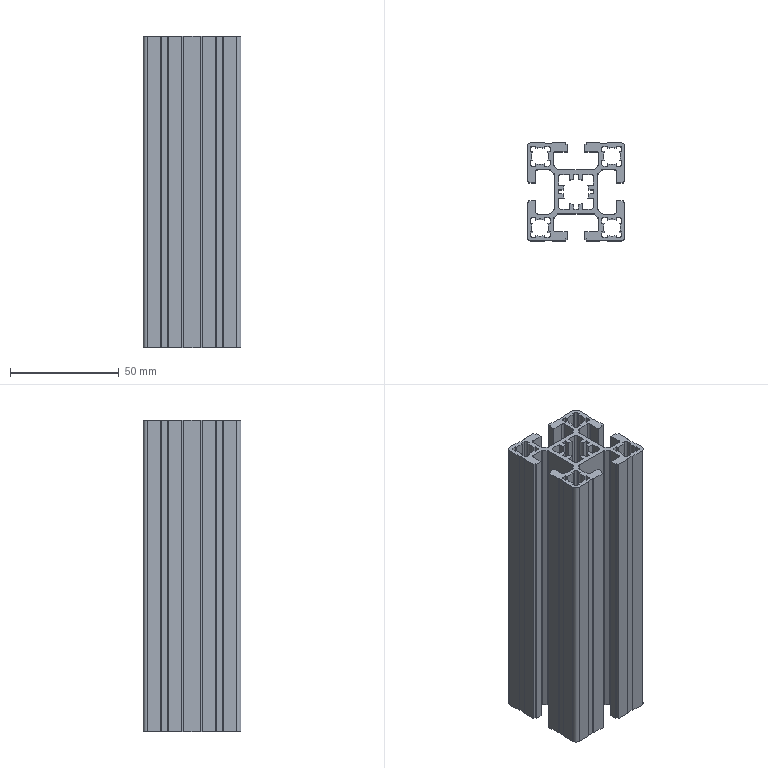Part | STEP file | 4545 profile NG mount 2 | 1 solid | 262 faces | box 45 x 45 x 143 mm | volume 99220 mm3 | plane 186 | cylinder 76 | commonest cylinder face diameters 2 x44 8 x20 12 x8 4 x4